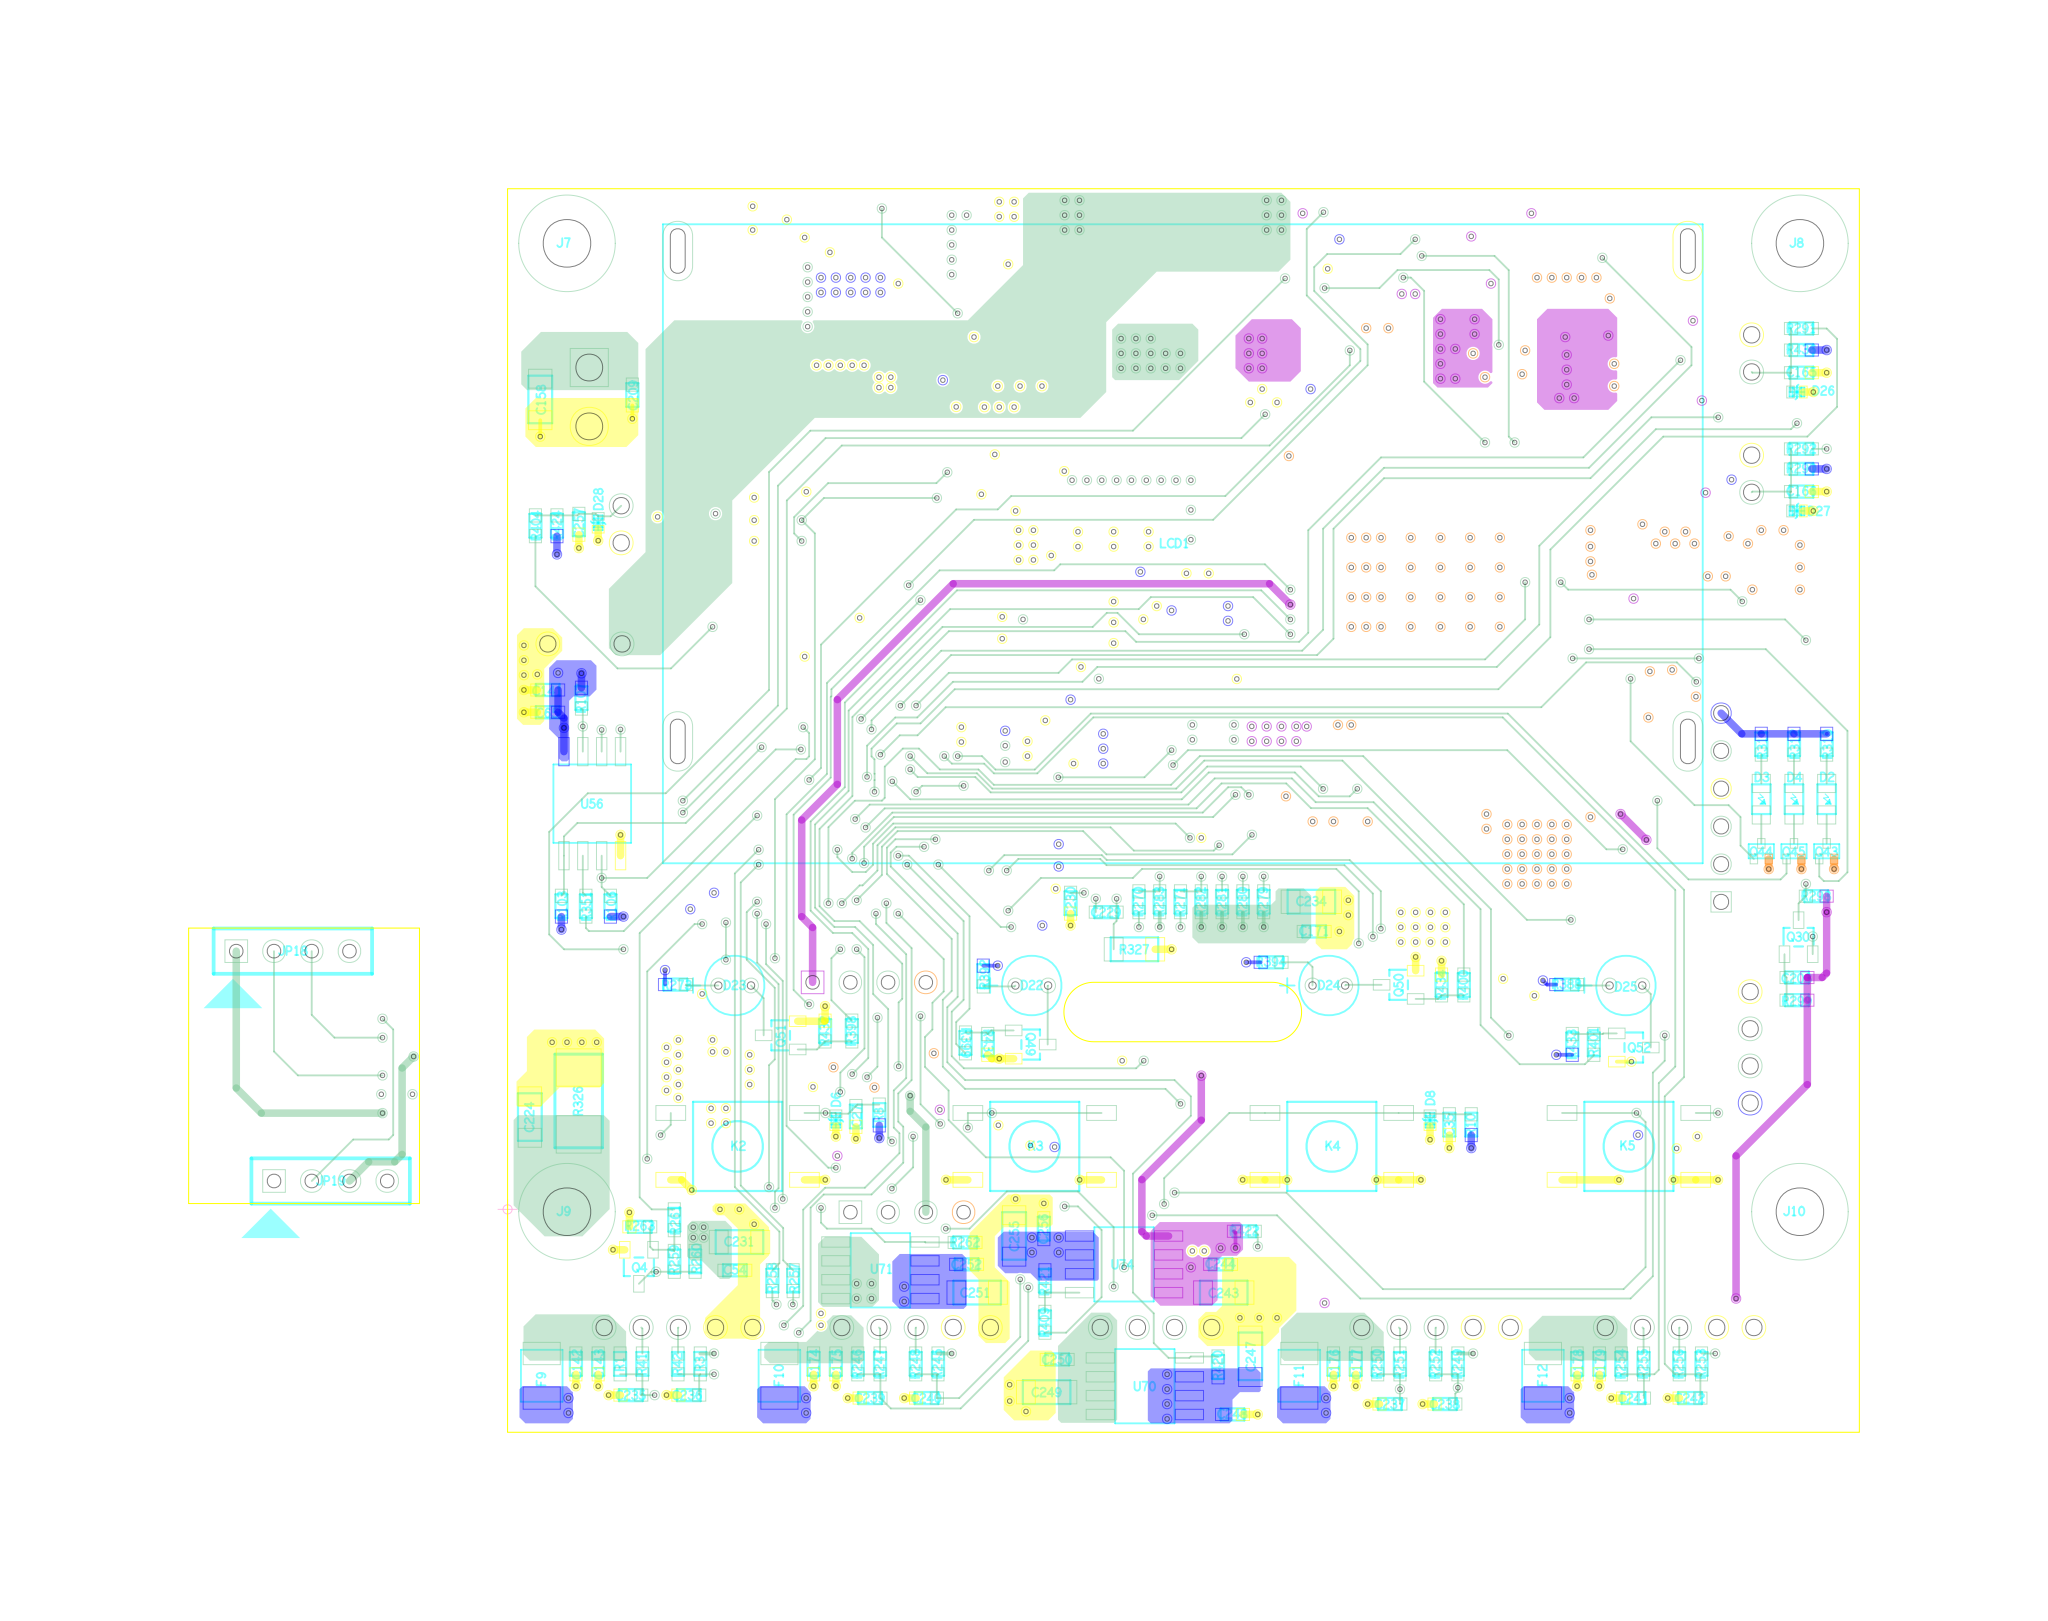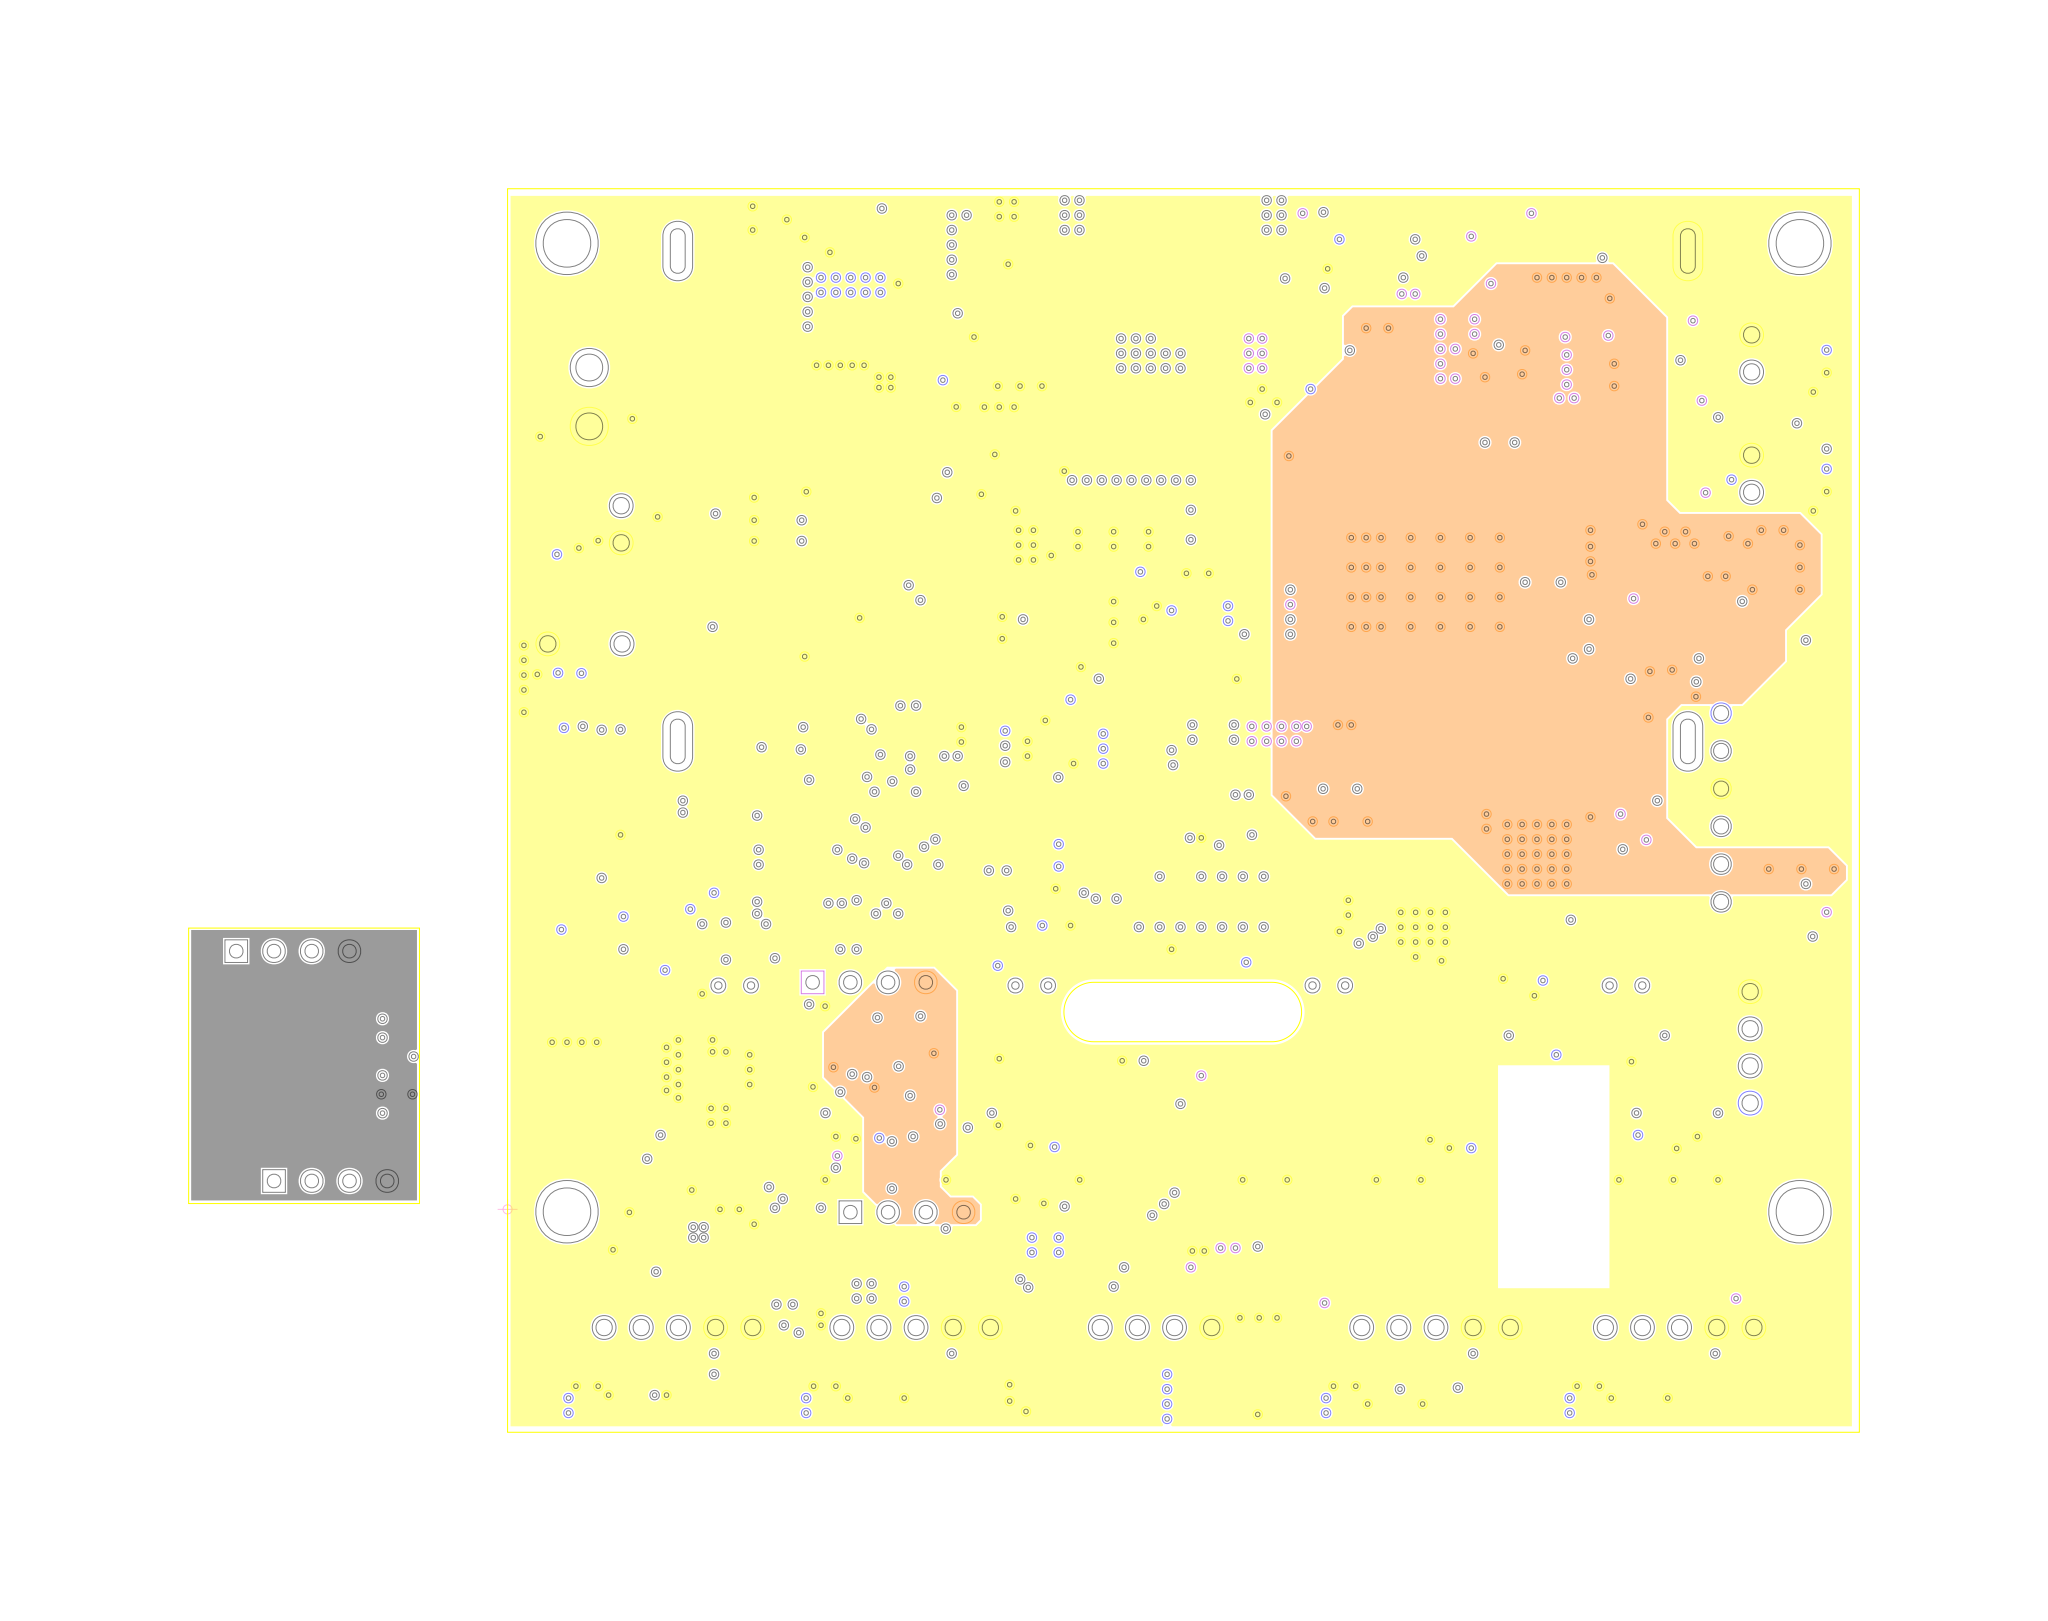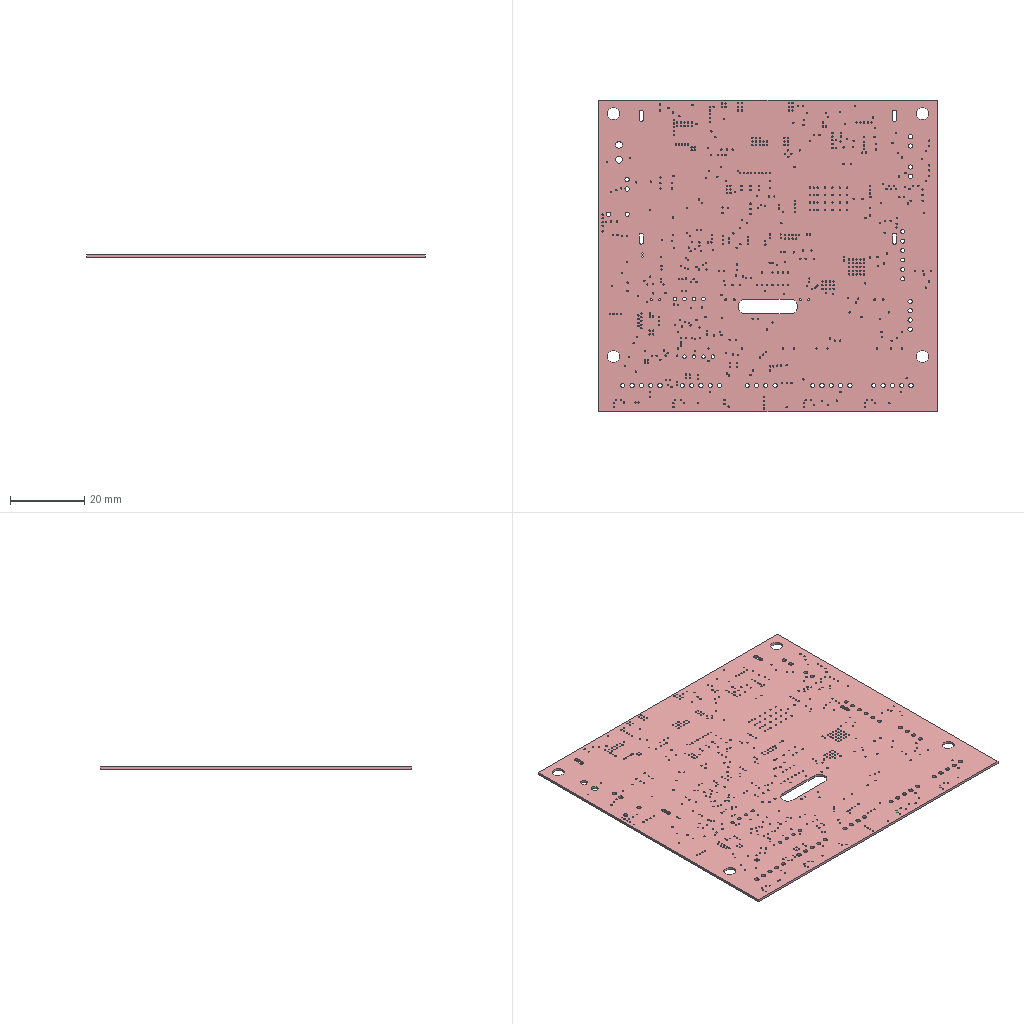Circuit board layout | Cadence Allegro | box 91 x 83.7 x 0.7 mm
Layer stack:
# Cadence Allegro layer stack of  (unit mm; from the constraint file cross-section; dielectric type: 0 not recorded (Allegro does not mark core vs prepreg), 3 surface material)
index,name,kind,layer,copper_thickness_mm,dielectric_type,dielectric_thickness_mm,dielectric_material,dielectric_constant
0,Top Surface,other,,,,,,
1,TOP,copper,TOP,0.0305,,,,
2,Dielectric1,dielectric,,,0,0.2032,FR-4,4.5
3,L2_GND,copper,L2_GND,0.0305,,,,
4,Dielectric2,dielectric,,,0,0.2032,FR-4,4.5
5,L3_PWR,copper,L3_PWR,0.0305,,,,
6,Dielectric3,dielectric,,,0,0.2032,FR-4,4.5
7,BOTTOM,copper,BOTTOM,0.0305,,,,
8,Bottom Surface,other,,,,,,
# drill layer pairs: low layer,high layer
drill_pair,TOP,BOTTOM
Part placement:
REFDES,COMP_VALUE,SYM_NAME,SYM_X,SYM_Y,SYM_ROTATE,SYM_MIRROR
C6,,C0603,47.2,41.1,270.000,YES
C7,,C0603,35.5,33.9,180.000,YES
C10,,C0603,31.7,38.4,180.000,YES
C26,,C0603,78.7,5.7,90.000,YES
C27,,C0603,23.45,6.252,270.000,NO
C34,,C0603,35.2,5.952,90.000,YES
C35,,C0603,63.4,5.7,270.000,NO
C54,,C0603,15.3,-4.1,0.000,NO
C63,,C0603,45.7,41.1,270.000,YES
C64,,C0603,43.7,42.2,90.000,YES
C65,,C0603,2.702,33.45,180.000,NO
C81,,C0603,33,57.1,90.000,YES
C141,,C0603,2.702,34.95,180.000,NO
C142,,C0603,4.6,-10.4,270.000,NO
C143,,C0603,6.1,-10.4,270.000,NO
C153,,C0603,59.346,60.917,90.000,YES
C154,,C0603,57.846,60.917,90.000,YES
C155,,C0603,51.746,59.017,90.000,YES
C156,,C0603,53.246,59.017,90.000,YES
C158,,C1206,2.2,54.5,270.000,NO
C165,,C0603,87.1,56.3,0.000,NO
C166,,C0603,87.102,48.3,0.000,NO
C171,,C0603,54.3,18.7,0.000,NO
C173,,C0603,38.8,29.1,0.000,YES
C174,,C0603,20.6,-10.4,270.000,NO
C175,,C0603,22.1,-10.4,270.000,NO
C176,,C0603,55.6,-10.4,270.000,NO
C177,,C0603,57.1,-10.4,270.000,NO
C178,,C0603,72,-10.4,270.000,NO
C179,,C0603,73.5,-10.4,270.000,NO
C180,,C0603,22.4,38.6,0.000,YES
C181,,C0603,19.3,38.6,180.000,YES
C182,,C0603,35.3,21.575,180.000,YES
C183,,C0603,37.9,35.347,180.000,YES
C184,,C0603,37.9,37.847,180.000,YES
C185,,C0603,39.1,39.5,180.000,YES
C186,,C0603,40.8,36.4,270.000,YES
C187,,C0603,64.378,55.171,180.000,YES
C188,,C0603,72.9,56.9,180.000,YES
C189,,C0603,72.9,55.4,180.000,YES
C190,,C0603,69.7,56.9,0.000,YES
C191,,C0603,69.7,55.4,0.000,YES
C192,,C0603,64.378,56.695,180.000,YES
C193,,C0603,80.8,44.395,270.000,YES
C194,,C0603,76.4,44.395,270.000,YES
C195,,C0603,24.9,11.2,90.000,YES
C196,,C0603,27.8,11.2,90.000,YES
C197,,C0603,24.5,3,270.000,YES
C198,,C0603,21.937,11.21,90.000,YES
C199,,C0603,53.4,29.3,180.000,YES
C200,,C0603,76.8,34.6,270.000,YES
C201,,C0603,56.5,29.3,0.000,YES
C202,,C0603,76.9,37.7,270.000,YES
C203,,C0603,86.802,15.6,180.000,NO
C204,,C0603,76.8,40.8,90.000,YES
C205,,C0603,78.6,46.8,0.000,YES
C206,,C0603,62.698,61.6,180.000,YES
C207,,C0603,78.002,59.8,0.000,YES
C208,,C0603,67.2,65.5,0.000,YES
C209,,C0603,8.4,54.8,270.000,NO
C210,,C0603,32.1,63.6,180.000,YES
C211,,C0603,21.5,58.8,90.000,YES
C213,,C1206,32.411,65.6,180.000,YES
C214,,C1206,31.712,52.7,180.000,YES
C215,,C1206,28.2,59.188,90.000,YES
C216,,C1206,25.8,59.188,90.000,YES
C217,,C1206,39.6,46.589,90.000,YES
C218,,C1206,37.2,46.589,90.000,YES
C219,,C0603,27.9,62.3,180.000,YES
C220,,C0603,34.5,57.1,270.000,YES
C221,,C0603,26.8,55.298,270.000,YES
C222,,C0603,31.2,50.7,180.000,YES
C223,,C0603,35.1,47.4,90.000,YES
C224,,C1206,1.5,6.211,90.000,NO
C225,,C1206,72.4,60.111,270.000,YES
C226,,C1206,70,60.111,270.000,YES
C227,,C1206,36.2,41.111,270.000,YES
C228,,C1206,42.8,37.111,270.000,YES
C229,,C0603,40.3,20,180.000,NO
C230,,C0603,37.9,20.6,270.000,NO
C231,,C1206,15.611,-2.2,0.000,NO
C232,,C1206,47.7,37.089,90.000,YES
C233,,C1206,37.589,31.2,0.000,YES
C234,,C1206,54.111,20.7,0.000,NO
C235,,C0603,8.3,-12.5,180.000,NO
C236,,C0603,12.2,-12.5,180.000,NO
C237,,C0603,59.4,-13.1,180.000,NO
C238,,C0603,63.1,-13.1,180.000,NO
C239,,C0603,24.4,-12.7,180.000,NO
C240,,C0603,28.2,-12.7,180.000,NO
C241,,C0603,75.8,-12.7,180.000,NO
C242,,C0603,79.6,-12.7,180.000,NO
C243,,C1206,48.212,-5.6,0.000,NO
C244,,C0603,48,-3.7,0.000,NO
C247,,C1206,50,-9.889,90.000,NO
C248,,C0603,48.8,-13.8,0.000,NO
C249,,C1206,36.288,-12.3,180.000,NO
C250,,C0603,37,-10.1,180.000,NO
C251,,C1206,31.611,-5.6,0.000,NO
C252,,C0603,30.9,-3.7,0.000,NO
C255,,C1206,34.1,-1.788,90.000,NO
C256,,C0603,36.1,-1.3,90.000,NO
C257,,C0603,4.8,46.1,270.000,NO
C259,,C1206,21.3,54.312,270.000,YES
C260,,C1206,23.7,54.312,270.000,YES
C261,,C1206,21.3,49.688,90.000,YES
C262,,C1206,42,46.589,90.000,YES
C263,,C1206,44.3,46.589,90.000,YES
C264,,C1206,18.8,64.011,270.000,YES
C265,,C1206,23.4,59.189,90.000,YES
C266,,DE10MM,5.209,38.052,270.000,YES
C267,,C0603,12.1,48.2,0.000,YES
C268,,C0603,18.3,47.9,0.000,YES
C269,,C0603,21,66,90.000,YES
C270,,C0603,52.546,56.717,0.000,YES
C271,,C0603,52.546,55.217,0.000,YES
D2,,LED0805,88.8,27.6,270.000,NO
D3,,LED0805,84.4,27.6,270.000,NO
D4,,LED0805,86.6,27.6,270.000,NO
D5,,SMA,14.998,64.8,90.000,YES
D6,,DFN1006-2,22.1,6,90.000,NO
D7,,DFN1006-2,33.8,6.1,270.000,YES
D8,,DFN1006-2,62.1,6,90.000,NO
D9,,DFN1006-2,80.1,6,270.000,YES
D10,,DFN1006-2,12.162,6.5,180.000,YES
D11,,DFN1006-2,82.2,44.134,90.000,YES
D20,,SMB,47.85,48,270.000,YES
D21,,SMB,47.85,55.1,270.000,YES
D22,,LED1,35.287,15.063,0.000,NO
D23,,LED1,15.287,15.063,0.000,NO
D24,,LED1,55.287,15.063,0.000,NO
D25,,LED1,75.287,15.063,0.000,NO
D26,,DFN1006-2,86.8,55,180.000,NO
D27,,DFN1006-2,86.8,47,180.000,NO
D28,,DFN1006-2,6.1,46.2,90.000,NO
D29,,DFN1006-2,74.2,60.1,90.000,YES
F9,,1210,2.3,-11.2,90.000,NO
F10,,1210,18.3,-11.2,90.000,NO
F11,,1210,53.3,-11.2,90.000,NO
F12,,1210,69.7,-11.2,90.000,NO
F13,,FUSE_798X544,15.3,58.2,0.000,YES
F14,,FUSE_798X544,15.3,52.1,0.000,YES
F15,,FUSE_798X544,41.6,63.6,90.000,YES
F16,,FUSE_798X544,47.8,63.6,270.000,YES
J3,,D1AX2N-3_96MM-VH,5.5,56.648,270.000,YES
J4,,HEADER_1X6_ANGLED,81.695,20.69,90.000,YES
J7,,MT0-3_2-6_5MM,4,65.005,0.000,NO
J8,,MT0-3_2-6_5MM,87,65.005,0.000,NO
J9,,MT0-3_2-6_5MM,4,-0.1593,0.000,NO
J10,,MT0-3_2-6_5MM,87,-0.1593,0.000,NO
J11,,MN-305-ARP7,-14.1,9.65,270.000,YES
J13,,HX_XHB2_54-2AW,83.75,57.6,270.000,YES
J14,,HX_XHB2_54-2AW,83.75,49.5,270.000,YES
J15,,FPC_05_20_XC,45.86,24.225,0.000,YES
J16,,HX_XHB2_54-2AW,7.65,46.1,90.000,YES
JP8,,KH-IPEX-K501-29,85.4,43.2,270.000,YES
JP9,,HX_XHB2_54-5AW,11.5,-7.95,180.000,YES
JP10,,HX_XHB2_54-5AW,27.5,-7.95,180.000,YES
JP11,,HX_XHB2_54-5AW,62.5,-7.95,180.000,YES
JP12,,HX_XHB2_54-5AW,78.9,-7.95,180.000,YES
JP13,,KH-IPEX-K501-29,12.6,13,0.000,YES
JP14,,HX_XHB2_54-4AW,44.9,-7.95,180.000,YES
JP15,,HX_XHB2_54-4AW,83.65,12.15,270.000,YES
JP16,,D1AX4N-2_54MM,24.345,15.275,180.000,YES
JP17,,D1AX4N-2_54MM,26.889,-0.1914,180.000,YES
JP18,,D1AX4N-2_54MM,-14.455,17.375,0.000,NO
JP19,,D1AX4N-2_54MM,-11.911,1.909,0.000,NO
K2,,ZX-QC66-65TP,15.486,4.235,0.000,NO
K3,,ZX-QC66-65TP,35.486,4.235,0.000,NO
K4,,ZX-QC66-65TP,55.486,4.235,0.000,NO
K5,,ZX-QC66-65TP,75.486,4.235,0.000,NO
L3,,L-4X4-IND_1UH_4A_MC,35.905,61.025,90.000,YES
L5,,IND_4R7UH_10A5,26.4,48.4,180.000,YES
L6,,IND_1008,13.745,8.8,0.000,YES
LCD1,,LCD_70X43X6,45.456,44.788,0.000,NO
Q2,,SOT_23_IRLML6402,14.015,45.856,270.000,YES
Q4,,SOT23-123-095,8.84,-3.865,180.000,NO
Q30,,SOT23-123-095,86.91,18.315,0.000,NO
Q31,,SOT23-123-095,78.01,57.185,180.000,YES
Q32,,SOT23-123-095,67.41,62.885,180.000,YES
Q33,,SOT23-123-095,81.015,40.91,270.000,YES
Q34,,SOT23-123-095,78.715,50.51,270.000,YES
Q35,,SOT23-123-095,62.49,64.215,0.000,YES
Q39,,SOT_416FL,57.4,27.4,90.000,YES
Q40,,SOT_416FL,78.9,37.6,0.000,YES
Q41,,SOT_416FL,55.1,27.4,90.000,YES
Q42,,SOT_416FL,78.7,35,90.000,YES
Q43,,SOT_416FL,88.8,24.1,0.000,NO
Q44,,SOT_416FL,84.4,24.1,0.000,NO
Q45,,SOT_416FL,86.6,24.1,0.000,NO
Q49,,SOT23-123-095,35.215,11.09,270.000,NO
Q50,,SOT23-123-095,59.985,15.11,90.000,NO
Q51,,SOT23-123-095,18.385,11.71,90.000,NO
Q52,,SOT23-123-095,75.815,10.89,270.000,NO
Q53,,TO252-134,69.3,17.4,0.000,YES
Q54,,SOT23-123-095,19.61,8.085,180.000,YES
Q55,,SOT_23_IRLML6402,55.69,57.832,0.000,YES
R1,,R0603,7.575,-10.4,90.000,NO
R2,,R0603,77.125,5.7,270.000,YES
R3,,R0603,12.975,-10.4,90.000,NO
R8,,R0603,25.025,6.35,90.000,NO
R9,,R0603,36.825,5.85,270.000,YES
R10,,R0603,64.875,5.7,90.000,NO
R41,,R0603,9.075,-10.4,90.000,NO
R42,,R0603,11.475,-10.4,90.000,NO
R70,,R1206,28.3,65.4,90.000,YES
R74,,R0603,28.275,55.3,90.000,YES
R101,,R1206,45.2,37.1,90.000,YES
R102,,R1206,39.9,42.9,0.000,YES
R103,,R0603,3.625,20.4,270.000,NO
R106,,R0603,6.925,20.4,270.000,NO
R107,,R0603,4.975,34.4,90.000,NO
R132,,R0603,35.8,52.575,180.000,YES
R134,,R0603,35.8,51.125,0.000,YES
R135,,R0603,35.8,49.675,180.000,YES
R136,,R0603,78.5,43.697,0.000,YES
R245,,R0603,28.975,-10.4,90.000,NO
R246,,R0603,23.575,-10.4,90.000,NO
R247,,R0603,25.075,-10.4,90.000,NO
R248,,R0603,27.475,-10.4,90.000,NO
R249,,R0603,63.975,-10.4,90.000,NO
R250,,R0603,58.575,-10.4,90.000,NO
R251,,R0603,60.075,-10.4,90.000,NO
R252,,R0603,62.475,-10.4,90.000,NO
R253,,R0603,80.375,-10.4,90.000,NO
R254,,R0603,74.975,-10.4,90.000,NO
R255,,R0603,76.475,-10.4,90.000,NO
R256,,R0603,78.875,-10.4,90.000,NO
R257,,R0603,19.225,-4.8,270.000,NO
R258,,R0603,17.825,-4.8,270.000,NO
R259,,R0603,11.225,-3.5,270.000,NO
R260,,R0603,12.625,-3.5,270.000,NO
R261,,R0603,11.225,-0.7,270.000,NO
R262,,R0603,30.8,-2.225,180.000,NO
R263,,R0603,8.9,-1.175,0.000,NO
R270,,R0603,42.5,20.7,90.000,NO
R271,,R0603,45.3,20.7,90.000,NO
R273,,R0603,11.3,15.125,0.000,NO
R276,,R0603,35.3,23.075,180.000,YES
R277,,R0603,35.3,24.575,180.000,YES
R278,,R0603,35.3,20.1,180.000,YES
R279,,R0603,50.9,20.7,90.000,NO
R280,,R0603,49.5,20.7,90.000,NO
R281,,R0603,48.1,20.7,90.000,NO
R282,,R0603,46.7,20.7,90.000,NO
R283,,R0603,43.9,20.7,90.000,NO
R284,,R0603,38.6,33.325,0.000,YES
R285,,R0603,39.1,40.9,180.000,YES
R286,,R0603,11.075,45.9,90.000,YES
R287,,R0603,31.7,41.375,180.000,YES
R288,,R0603,31.7,39.875,180.000,YES
R290,,R0603,87.1,49.825,0.000,NO
R291,,R0603,87.1,59.275,180.000,NO
R292,,R0603,87.1,51.175,180.000,NO
R294,,R0603,23.075,2.9,90.000,YES
R295,,R0603,23.425,11.2,270.000,YES
R296,,R0603,26.325,11.2,270.000,YES
R297,,R0603,25.875,3,90.000,YES
R298,,R0603,88.1,21.075,180.000,NO
R299,,R0603,86.8,14.075,180.000,NO
R300,,R0603,78.6,54.425,0.000,YES
R301,,R0603,78,61.225,0.000,YES
R302,,R0603,66.9,60.275,180.000,YES
R303,,R0603,67.2,67.025,0.000,YES
R304,,R0603,78.375,40.8,90.000,YES
R305,,R0603,84.7,40.025,0.000,YES
R306,,R0603,78.6,48.225,0.000,YES
R307,,R0603,81.525,49.8,270.000,YES
R308,,R0603,64.875,63.8,90.000,YES
R309,,R0603,59.3,65.275,180.000,YES
R310,,R0603,88.8,31.3,270.000,NO
R311,,R0603,84.4,31.3,270.000,NO
R312,,R0603,86.6,31.3,270.000,NO
R313,,R0603,53.525,65.5,270.000,YES
R314,,R0603,27.275,3,90.000,YES
R315,,R0603,26.425,66,270.000,YES
R316,,R0603,30.125,57.1,270.000,YES
R318,,R0603,31.575,57.1,90.000,YES
R319,,R0603,30.9,54.925,0.000,YES
R320,,R0603,35.975,57.1,90.000,YES
R321,,R0603,18.3,46.375,180.000,YES
R322,,R0603,21.3,44.925,0.000,YES
R323,,R0603,18.3,44.975,180.000,YES
R324,,R0603,35.8,54.025,0.000,YES
R326,,R2512,4.787,7.294,90.000,NO
R327,,R1206,42.2,17.5,180.000,NO
R331,,R0603,31.625,18.2,270.000,YES
R332,,R0603,30.225,18.2,270.000,YES
R333,,R0603,26.025,18.2,270.000,YES
R334,,R0603,54.925,65.5,270.000,YES
R335,,R0603,58.646,63.142,0.000,YES
R336,,R0603,66.725,56.4,270.000,YES
R338,,R0603,27.425,18.2,270.000,YES
R342,,R0603,14.8,27.275,180.000,YES
R343,,R0603,14.8,25.775,180.000,YES
R344,,R0603,14.8,30.175,180.000,YES
R348,,R0603,14.8,33.075,180.000,YES
R349,,R0603,14.8,34.575,180.000,YES
R351,,R0603,5.275,20.4,90.000,NO
R352,,R0603,29.37,39.304,270.000,YES
R353,,R0603,27.795,39.304,270.000,YES
R354,,R0603,16.325,39.5,270.000,YES
R360,,R0603,35.3,29.075,180.000,YES
R369,,R0603,76.425,28.2,270.000,YES
R377,,R0603,35.3,26.075,180.000,YES
R378,,R0603,35.3,27.575,180.000,YES
R379,,R1206,62.6,59.4,180.000,YES
R380,,R0603,74.925,28.2,270.000,YES
R381,,R0603,73.475,28.2,90.000,YES
R382,,R0603,42.425,-3.2,270.000,YES
R385,,R0603,42.825,8.3,270.000,YES
R386,,R0603,24.625,18.2,270.000,YES
R388,,R0603,71.3,15.125,0.000,NO
R391,,R0603,43.925,-3.2,270.000,YES
R392,,R0603,32.025,15.7,270.000,NO
R394,,R0603,51.4,16.625,0.000,NO
R398,,R0603,23.175,12,90.000,NO
R399,,R0603,30.825,11.2,270.000,NO
R400,,R0603,64.375,15.1,90.000,NO
R401,,R0603,73.125,11.1,270.000,NO
R404,,R0603,1.875,46,90.000,NO
R406,,R0603,14.8,31.575,180.000,YES
R409,,R0603,36.175,-7.6,90.000,NO
R410,,R0603,21.3,46.375,180.000,YES
R411,,R2010,60.3,23.7,90.000,YES
R412,,R2010,63.8,23.7,90.000,YES
R413,,R2010,40.5,52.6,270.000,YES
R414,,R2010,43.9,52.6,270.000,YES
R420,,R0603,47.825,-10.6,270.000,NO
R421,,R0603,36.175,-4.8,90.000,NO
R422,,R0603,49.6,-1.475,0.000,NO
R423,,R0603,41.375,8.3,90.000,YES
R424,,R0603,3.325,46,270.000,NO
R427,,R0603,26.351,39.3,270.000,YES
R428,,R0603,24.825,39.3,270.000,YES
R429,,R0603,80.9,9.725,0.000,YES
R430,,R0603,28.825,18.2,270.000,YES
R431,,R0603,32.325,11.1,270.000,NO
R432,,R0603,21.375,12,90.000,NO
R433,,R0603,71.675,11.1,90.000,NO
R434,,R0603,62.875,15.1,90.000,NO
R435,,R0603,70.6,14.375,180.000,YES
R436,,R0603,87.1,57.825,0.000,NO
R437,,R0603,44.275,8.3,90.000,YES
R438,,R0603,19.6,12.175,180.000,YES
R439,,R0603,19.6,10.625,0.000,YES
R440,,R0603,17.325,8.3,270.000,YES
R441,,R0603,55.646,55.142,0.000,YES
R442,,R0603,14.8,28.775,180.000,YES
TP1,,TPC30-75,60.6,28.3,270.000,YES
TP2,,TPC30-75,62.6,28.3,270.000,YES
TP3,,TPC30-75,60.4,56.2,270.000,YES
TP4,,TPC30-75,58.4,56.2,270.000,YES
U1,,LQFP80,25.25,28.7,270.000,YES
U24,,SO8,44.55,31.3,180.000,YES
U56,,SOB_8_208MIL,5.7,27.3,90.000,NO
U59,,EC600K-CN,62.797,42.197,270.000,YES
U60,,SOT23-6L,27,6.7,270.000,YES
U64,,SOT-23A-3,23.7,66,0.000,YES
U66,,QFN2X3-13,32,60.8,180.000,YES
U67,,DFN3X3_12,31.897,48.119,180.000,YES
U68,,TAU1113,15.9,-0.3,90.000,YES
U70,,SO8,42.9,-11.9,180.000,NO
U71,,SO8,25.1,-4.1,180.000,NO
U74,,SO8,41.5,-3.7,0.000,NO
U75,,BLUETEETH_JDY-31,59.177,2.194,270.000,YES
U76,,SOT23-8,54.846,62.317,270.000,YES
Y2,,OSC_3215,35.155,36.597,90.000,YES
Y4,,XTAL_5032_4P,20.4,41.4,0.000,YES
Pad and via stacks:
# Allegro (Cadence) via spans and padstacks; design units: ("millimeters" 4 10000)
# via spans: padstack,start_layer,end_layer,net_example,count
VIA12-BGA,ETCH/TOP,ETCH/BOTTOM,CON_VDD,667
# Allegro padstack definitions: name,start_layer,end_layer,drill,plating,holeType,type
SMD2P5X1P5,"ETCH/TOP","ETCH/TOP",0.0,"PLATED","none","smd"
SMD0P8X0P5,"ETCH/TOP","ETCH/TOP",0.0,"PLATED","none","smd"
OBL1_80X0_70,"ETCH/TOP","ETCH/TOP",0.0,"PLATED","none","smd"
OBL0_70X1_80,"ETCH/TOP","ETCH/TOP",0.0,"PLATED","none","smd"
SQU1_00,"ETCH/TOP","ETCH/TOP",0.0,"PLATED","none","smd"
SMD2P0X3P0,"ETCH/TOP","ETCH/TOP",0.0,"PLATED","none","smd"
SMD0P3X1P7,"ETCH/TOP","ETCH/TOP",0.0,"PLATED","none","smd"
SMD1P1X2P6,"ETCH/TOP","ETCH/TOP",0.0,"PLATED","none","smd"
SMDS1P0,"ETCH/TOP","ETCH/TOP",0.0,"PLATED","none","smd"
SMD2P2X1P0,"ETCH/TOP","ETCH/TOP",0.0,"PLATED","none","smd"
SMD0P3X1P5,"ETCH/TOP","ETCH/TOP",0.0,"PLATED","none","smd"
SMD0P9X1P35,"ETCH/TOP","ETCH/TOP",0.0,"PLATED","none","smd"
SMD1P3X1P8,"ETCH/TOP","ETCH/TOP",0.0,"PLATED","none","smd"
SMD0P7X1P9,"ETCH/TOP","ETCH/TOP",0.0,"PLATED","none","smd"
SMD0P4X0P8,"ETCH/TOP","ETCH/TOP",0.0,"PLATED","none","smd"
SMD1P06X0P65,"ETCH/TOP","ETCH/TOP",0.0,"PLATED","none","smd"
SMD1P2X0P8,"ETCH/TOP","ETCH/TOP",0.0,"PLATED","none","smd"
SMD0P75X1P8,"ETCH/TOP","ETCH/TOP",0.0,"PLATED","none","smd"
SMD0P3X0P85,"ETCH/TOP","ETCH/TOP",0.0,"PLATED","none","smd"
SMD1P0X2P0,"ETCH/TOP","ETCH/TOP",0.0,"PLATED","none","smd"
SMD0P25X0P56,"ETCH/TOP","ETCH/TOP",0.0,"PLATED","none","smd"
SMD0P25X1P0,"ETCH/TOP","ETCH/TOP",0.0,"PLATED","none","smd"
SMDS0P7,"ETCH/TOP","ETCH/TOP",0.0,"PLATED","none","smd"
C5,"ETCH/TOP","ETCH/TOP",0.0,"PLATED","none","smd"
SMD35X32,"ETCH/TOP","ETCH/TOP",0.0,"PLATED","none","smd"
SMD50X62,"ETCH/TOP","ETCH/TOP",0.0,"PLATED","none","smd"
SMD57X166,"ETCH/TOP","ETCH/TOP",0.0,"PLATED","none","smd"
SMD48X48,"ETCH/TOP","ETCH/TOP",0.0,"PLATED","none","smd"
SMD100X75,"ETCH/TOP","ETCH/TOP",0.0,"PLATED","none","smd"
SMD99X119,"ETCH/TOP","ETCH/TOP",0.0,"PLATED","none","smd"
SMD67X99,"ETCH/TOP","ETCH/TOP",0.0,"PLATED","none","smd"
SMD24X39,"ETCH/TOP","ETCH/TOP",0.0,"PLATED","none","smd"
SMD28X44,"ETCH/TOP","ETCH/TOP",0.0,"PLATED","none","smd"
TPC30-75,"ETCH/TOP","ETCH/TOP",0.0,"PLATED","none","smd"
SMD0P3X0P75,"ETCH/TOP","ETCH/TOP",0.0,"PLATED","none","smd"
SMD2P7X1P7,"ETCH/TOP","ETCH/TOP",0.0,"PLATED","none","smd"
SMD44X71,"ETCH/TOP","ETCH/TOP",0.0,"PLATED","none","smd"
THC1P6D1P1,"ETCH/TOP","ETCH/BOTTOM",1.1,"PLATED","circle_drill","through"
THO4P0X2P0D3P0X1P0,"ETCH/TOP","ETCH/BOTTOM",1.0,"PLATED","oval slot","through"
C101D71,"ETCH/TOP","ETCH/BOTTOM",1.803,"PLATED","circle_drill","through"
S101D71,"ETCH/TOP","ETCH/BOTTOM",1.803,"PLATED","circle_drill","through"
S54D40,"ETCH/TOP","ETCH/BOTTOM",1.016,"PLATED","circle_drill","through"
C54D40,"ETCH/TOP","ETCH/BOTTOM",1.016,"PLATED","circle_drill","through"
PAD6_5CIR3_2D-MM,"ETCH/TOP","ETCH/BOTTOM",3.2,"PLATED","circle_drill","through"
C54D35,"ETCH/TOP","ETCH/BOTTOM",0.889,"PLATED","circle_drill","through"
VIA12-BGA,"ETCH/TOP","ETCH/BOTTOM",0.3048,"PLATED","circle_drill","through"
SMD1P4X1P2,"ETCH/TOP","ETCH/TOP",0.0,"PLATED","none","smd"
SMD2P5X2P3,"ETCH/TOP","ETCH/TOP",0.0,"PLATED","none","smd"
SMD1P4X2P8,"ETCH/TOP","ETCH/TOP",0.0,"PLATED","none","smd"
SMD6P20X5P8,"ETCH/TOP","ETCH/TOP",0.0,"PLATED","none","smd"
SMD2P3X1P0,"ETCH/TOP","ETCH/TOP",0.0,"PLATED","none","smd"
THC1P0D0P5,"ETCH/TOP","ETCH/BOTTOM",0.5,"PLATED","circle_drill","through"
SMD2P3X5P3,"ETCH/TOP","ETCH/TOP",0.0,"PLATED","none","smd"
SMD1P3X5P2,"ETCH/TOP","ETCH/TOP",0.0,"PLATED","none","smd"
SMD0P65X0P5,"ETCH/TOP","ETCH/TOP",0.0,"PLATED","none","smd"
SMD1P5X3P0,"ETCH/TOP","ETCH/TOP",0.0,"PLATED","none","smd"
SMD0P4X1P2,"ETCH/TOP","ETCH/TOP",0.0,"PLATED","none","smd"
SMD1P2X1P7,"ETCH/TOP","ETCH/TOP",0.0,"PLATED","none","smd"
S60D36,"ETCH/TOP","ETCH/BOTTOM",0.9144,"PLATED","circle_drill","through"
C60D36,"ETCH/TOP","ETCH/BOTTOM",0.9144,"PLATED","circle_drill","through"
Design rules, without the lines most boards share, first 13 of 25 lines:
# Cadence Allegro design rules of  (from the Constraint Manager export constraints.dcfx, design unit mm; typed fields in mm)
# columns: name | kind | enabled | priority | scope1 | scope2 | descriptor | typed fields (field=value)
# Allegro precedence (priority 1 wins): 1 Region class-to-class, 2 Region class, 3 Region, 4 class-to-class, 5 DiffPair/Bus/NetGroup override, 6 NetClass, 7 constraint set (CSet) default
# per-layer values are written LAYER=value in the descriptor and LAYER:mm in the typed field; a maximum of 0 means no limit set
# --- net classes (and buses / net groups) ---
PWR | NetClass | enabled | 6 | GND, P3V3, P3V8, VBAT+, N00347, P3V3_LCD, VDD_EXT, USIM_VDD, VREFP, VRTC, GND_EARTH, GND_SIGNAL, N00283, N204409, P3V3_BT, N00397 | All | Net Class (PhysicalCSet=PWR) (members: 16 Net) | physicalcset=PWR
# --- track widths, neck and differential-pair gap (physical constraint sets) ---
PWR | PhysicalCSet | enabled | 7 | NetClass(1): PWR | All | Physical Constraint (Min Line Width=0.254mm) (Max Line Width=0mm) (Min Neck Width=0.2mm) (Max Neck Length=0mm) (DiffPair Primary Gap=0mm) (DiffPair Neck Gap=0mm) (DiffPair Min Space=0mm) (DiffPair Coupled +Tol=0mm) (DiffPair Coupled -Tol=0mm) (Min BB Via Stagger=0.127mm) (Max BB Via Stagger=0mm) (T-junctions=ANYWHERE) (Pad-pad direct connect=ALL_ALLOWED) (Allowed vias=VIA12-BGA) | min_line_width=0.254 min_neck_width=0.2 min_bvia_stagger=0.127 max_bvia_stagger=0 ts_allowed=ANYWHERE diffp_primary_gap=0 diffp_neck_gap=0 max_line_width=0 maximum_neck_length=0 pad_pad_direct_connect=ALL_ALLOWED allow_on_etch_subclass=TRUE diffp_coupled_plus=0 diffp_coupled_minus=0 diffp_min_space=0 vias=VIA12-BGA
DEFAULT | PhysicalCSet | enabled | 7 | Design default | All | Physical Constraint (Min Line Width=0.127mm) (Max Line Width=0mm) (Min Neck Width=0.127mm) (Max Neck Length=0mm) (DiffPair Primary Gap=0mm) (DiffPair Neck Gap=0mm) (DiffPair Min Space=0mm) (DiffPair Coupled +Tol=0mm) (DiffPair Coupled -Tol=0mm) (Min BB Via Stagger=0.127mm) (Max BB Via Stagger=0mm) (T-junctions=ANYWHERE) (Pad-pad direct connect=ALL_ALLOWED) (Allowed vias=VIA12-BGA) | min_line_width=0.127 min_neck_width=0.127 min_bvia_stagger=0.127 max_bvia_stagger=0 ts_allowed=ANYWHERE diffp_primary_gap=0 diffp_neck_gap=0 max_line_width=0 maximum_neck_length=0 pad_pad_direct_connect=ALL_ALLOWED allow_on_etch_subclass=TRUE diffp_coupled_plus=0 diffp_coupled_minus=0 diffp_min_space=0 vias=VIA12-BGA
# --- clearances: line / pad / via / shape / hole (spacing constraint sets) ---
DEFAULT | SpacingCSet | enabled | 7 | Design default | All | Clearance Constraint (Line-Line=0.127mm) (Line-SMD Pad=0.127mm) (Line-Thru Pin=0.127mm) (Line-Via=0.127mm) (Line-Shape=0.127mm) (SMD Pad-SMD Pad=0.127mm) (Thru Pin-Thru Pin=0.127mm) (Thru Pin-SMD Pad=0.127mm) (SMD Pad-Via=0.127mm) (Thru Pin-Via=0.127mm) (Via-Via=0.127mm) (Shape-SMD Pad=0.127mm) (Shape-Thru Pin=0.127mm) (Shape-Via=0.127mm) (Shape-Shape=0.127mm) (Hole-Hole=0.2032mm) (Hole-Line=0.2032mm) (Hole-Shape=0.2032mm) (BB Via-BB Via=0.127mm) (uVia-uVia=0.127mm) | thrupin_to_thrupin_spacing=0.127 thrupin_to_smdpin_spacing=0.127 thrupin_to_thruvia_spacing=0.127 line_to_thrupin_spacing=0.127 thrupin_to_shape_spacing=0.127 smdpin_to_smdpin_spacing=0.127 smdpin_to_thruvia_spacing=0.127 line_to_smdpin_spacing=0.127 shape_to_smdpin_spacing=0.127 thruvia_to_thruvia_spacing=0.127 line_to_thruvia_spacing=0.127 shape_to_thruvia_spacing=0.127 line_to_line_spacing=0.127 line_to_shape_spacing=0.127 shape_to_shape_spacing=0.127 bbv_to_bbv_spacing=0.127 bbv_to_thrupin_spacing=0.127 bbv_to_smdpin_spacing=0.127 bbv_to_thruvia_spacing=0.127 bbv_to_line_spacing=0.127 bbv_to_shape_spacing=0.127 bbv_to_testpin_spacing=0.127 bbv_to_testvia_spacing=0.127 testpin_to_testpin_spacing=0.127 testpin_to_thrupin_spacing=0.127 smdpin_to_testpin_spacing=0.127 testpin_to_thruvia_spacing=0.127 testpin_to_testvia_spacing=0.127 line_to_testpin_spacing=0.127 shape_to_testpin_spacing=0.127 testvia_to_testvia_spacing=0.127 testvia_to_thrupin_spacing=0.127 smdpin_to_testvia_spacing=0.127 testvia_to_thruvia_spacing=0.127 line_to_testvia_spacing=0.127 shape_to_testvia_spacing=0.127 bondpad_to_bondpad_spacing=0.127 thrupin_to_bondpad_spacing=0.127 smdpin_to_bondpad_spacing=0.127 bondpad_to_thruvia_spacing=0.127 bondpad_to_line_spacing=0.127 bondpad_to_shape_spacing=0.127 bondpad_to_bbv_spacing=0.127 bondpad_to_testpin_spacing=0.127 bondpad_to_testvia_spacing=0.127 min_bvia_gap=0.127 hole_to_pin_spacing=0.2032 hole_to_via_spacing=0.2032 hole_to_line_spacing=0.2032 hole_to_shape_spacing=0.2032 hole_to_hole_spacing=0.2032 mvia_to_mvia_spacing=0.127 mvia_to_thrupin_spacing=0.127 mvia_to_smdpin_spacing=0.127 mvia_to_thruvia_spacing=0.127 mvia_to_bbv_spacing=0.127 mvia_to_line_spacing=0.127 mvia_to_shape_spacing=0.127 mvia_to_testpin_spacing=0.127 mvia_to_testvia_spacing=0.127 bondpad_to_mvia_spacing=0.127 bondpad_to_bondpad_diffp_spc=0.127
DEFAULT | SameNetSpacingCSet | enabled | 7 | Design default | All | Same-Net Clearance (Line-Line=0.127mm) (Line-SMD Pad=0.127mm) (Line-Thru Pin=0.127mm) (Line-Via=0.127mm) (Line-Shape=0.127mm) (SMD Pad-SMD Pad=0.127mm) (Thru Pin-Thru Pin=0.127mm) (Thru Pin-SMD Pad=0.127mm) (SMD Pad-Via=0.127mm) (Thru Pin-Via=0.127mm) (Via-Via=0.127mm) (Shape-SMD Pad=0.127mm) (Shape-Thru Pin=0.127mm) (Shape-Via=0.127mm) (Shape-Shape=0.127mm) (Hole-Hole=0.2032mm) (Hole-Line=0.2032mm) (Hole-Shape=0.2032mm) (BB Via-BB Via=0.127mm) (uVia-uVia=0.127mm) | sn_thrupin_to_thrupin_spacing=0.127 sn_thrupin_to_smdpin_spacing=0.127 sn_thrupin_to_thruvia_spacing=0.127 sn_line_to_thrupin_spacing=0.127 sn_thrupin_to_shape_spacing=0.127 sn_smdpin_to_smdpin_spacing=0.127 sn_smdpin_to_thruvia_spacing=0.127 sn_line_to_smdpin_spacing=0.127 sn_shape_to_smdpin_spacing=0.127 sn_thruvia_to_thruvia_spacing=0.127 sn_line_to_thruvia_spacing=0.127 sn_shape_to_thruvia_spacing=0.127 sn_line_to_line_spacing=0.127 sn_line_to_shape_spacing=0.127 sn_shape_to_shape_spacing=0.127 sn_bbv_to_bbv_spacing=0.127 sn_bbv_to_thrupin_spacing=0.127 sn_bbv_to_smdpin_spacing=0.127 sn_bbv_to_thruvia_spacing=0.127 sn_bbv_to_line_spacing=0.127 sn_bbv_to_shape_spacing=0.127 sn_bbv_to_testpin_spacing=0.127 sn_bbv_to_testvia_spacing=0.127 sn_testpin_to_testpin_spacing=0.127 sn_testpin_to_thrupin_spacing=0.127 sn_smdpin_to_testpin_spacing=0.127 sn_testpin_to_thruvia_spacing=0.127 sn_testpin_to_testvia_spacing=0.127 sn_line_to_testpin_spacing=0.127 sn_shape_to_testpin_spacing=0.127 sn_testvia_to_testvia_spacing=0.127 sn_testvia_to_thrupin_spacing=0.127 sn_smdpin_to_testvia_spacing=0.127 sn_testvia_to_thruvia_spacing=0.127 sn_line_to_testvia_spacing=0.127 sn_shape_to_testvia_spacing=0.127 sn_bondpad_to_bondpad_spacing=0.127 sn_thrupin_to_bondpad_spacing=0.127 sn_smdpin_to_bondpad_spacing=0.127 sn_bondpad_to_thruvia_spacing=0.127 sn_bondpad_to_line_spacing=0.127 sn_bondpad_to_shape_spacing=0.127 sn_bondpad_to_bbv_spacing=0.127 sn_bondpad_to_testpin_spacing=0.127 sn_bondpad_to_testvia_spacing=0.127 same_net=TRUE sn_hole_to_pin_spacing=0.2032 sn_hole_to_via_spacing=0.2032 sn_hole_to_line_spacing=0.2032 sn_hole_to_shape_spacing=0.2032 sn_hole_to_hole_spacing=0.2032 sn_mvia_to_mvia_spacing=0.127 sn_mvia_to_thrupin_spacing=0.127 sn_mvia_to_smdpin_spacing=0.127 sn_mvia_to_thruvia_spacing=0.127 sn_mvia_to_bbv_spacing=0.127 sn_mvia_to_line_spacing=0.127 sn_mvia_to_shape_spacing=0.127 sn_mvia_to_testpin_spacing=0.127 sn_mvia_to_testvia_spacing=0.127 sn_bondpad_to_mvia_spacing=0.127
# --- differential pairs (0) ---